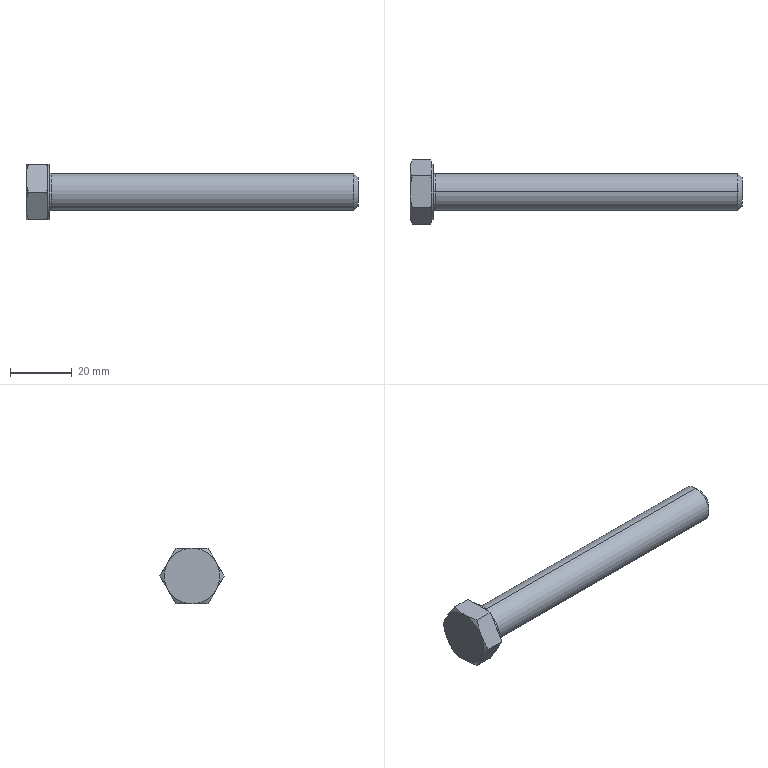Part | SolidWorks | features RevCut 4, Chamfer 1, Extrusion 1, Fillet 1, LPattern 1, Revolution 1 | 1 solid | 35 faces | box 107.5 x 20.785 x 18 mm | volume 13361 mm3 | plane 15 | cone 14 | cylinder 4 | torus 2 | commonest cylinder face diameters 12 x2 18 x2
STEP:
#1=CARTESIAN_POINT('',(8.1,0.,6.));
#2=VERTEX_POINT('',#1);
#3=CARTESIAN_POINT('',(8.1,0.,-6.));
#4=VERTEX_POINT('',#3);
#5=CARTESIAN_POINT('',(8.1,0.,0.));
#6=DIRECTION('',(1.,0.,0.));
#7=DIRECTION('',(0.,0.,-1.));
#8=AXIS2_PLACEMENT_3D('',#5,#6,#7);
#9=CIRCLE('',#8,6.);
#10=EDGE_CURVE('',#2,#4,#9,.T.);
#11=ORIENTED_EDGE('',*,*,#10,.F.);
#12=CARTESIAN_POINT('',(7.5,0.,6.6));
#13=VERTEX_POINT('',#12);
#14=CARTESIAN_POINT('',(8.1,0.,6.6));
#15=DIRECTION('',(0.,1.,0.));
#16=DIRECTION('',(0.,0.,1.));
#17=AXIS2_PLACEMENT_3D('',#14,#15,#16);
#18=CIRCLE('',#17,0.6);
#19=EDGE_CURVE('',#2,#13,#18,.T.);
#20=ORIENTED_EDGE('',*,*,#19,.T.);
#21=CARTESIAN_POINT('',(7.5,0.,-6.6));
#22=VERTEX_POINT('',#21);
#23=CARTESIAN_POINT('',(7.5,0.,0.));
#24=DIRECTION('',(-1.,0.,0.));
#25=DIRECTION('',(0.,0.,-1.));
#26=AXIS2_PLACEMENT_3D('',#23,#24,#25);
#27=CIRCLE('',#26,6.6);
#28=EDGE_CURVE('',#22,#13,#27,.T.);
#29=ORIENTED_EDGE('',*,*,#28,.F.);
#30=CARTESIAN_POINT('',(8.1,0.,-6.6));
#31=DIRECTION('',(0.,-1.,0.));
#32=DIRECTION('',(0.,0.,-1.));
#33=AXIS2_PLACEMENT_3D('',#30,#31,#32);
#34=CIRCLE('',#33,0.6);
#35=EDGE_CURVE('',#4,#22,#34,.T.);
#36=ORIENTED_EDGE('',*,*,#35,.F.);
#37=EDGE_LOOP('',(#11,#20,#29,#36));
#38=FACE_OUTER_BOUND('',#37,.T.);
#39=CARTESIAN_POINT('',(8.1,0.,0.));
#40=DIRECTION('',(1.,0.,0.));
#41=DIRECTION('',(0.,0.,-1.));
#42=AXIS2_PLACEMENT_3D('',#39,#40,#41);
#43=TOROIDAL_SURFACE('',#42,6.6,0.6);
#44=ADVANCED_FACE('',(#38),#43,.F.);
#45=CARTESIAN_POINT('',(107.5,0.,-4.6));
#46=VERTEX_POINT('',#45);
#47=CARTESIAN_POINT('',(107.5,0.,4.6));
#48=VERTEX_POINT('',#47);
#49=CARTESIAN_POINT('',(107.5,0.,0.));
#50=DIRECTION('',(1.,0.,0.));
#51=DIRECTION('',(0.,0.,1.));
#52=AXIS2_PLACEMENT_3D('',#49,#50,#51);
#53=CIRCLE('',#52,4.6);
#54=EDGE_CURVE('',#46,#48,#53,.T.);
#55=ORIENTED_EDGE('',*,*,#54,.F.);
#56=CARTESIAN_POINT('',(106.1,0.,-6.));
#57=VERTEX_POINT('',#56);
#58=CARTESIAN_POINT('',(106.1,0.,-6.));
#59=DIRECTION('',(-0.7071,0.,-0.7071));
#60=VECTOR('',#59,1000.);
#61=LINE('',#58,#60);
#62=EDGE_CURVE('',#46,#57,#61,.T.);
#63=ORIENTED_EDGE('',*,*,#62,.T.);
#64=CARTESIAN_POINT('',(106.1,0.,6.));
#65=VERTEX_POINT('',#64);
#66=CARTESIAN_POINT('',(106.1,0.,0.));
#67=DIRECTION('',(-1.,0.,0.));
#68=DIRECTION('',(0.,0.,1.));
#69=AXIS2_PLACEMENT_3D('',#66,#67,#68);
#70=CIRCLE('',#69,6.);
#71=EDGE_CURVE('',#65,#57,#70,.T.);
#72=ORIENTED_EDGE('',*,*,#71,.F.);
#73=CARTESIAN_POINT('',(106.1,0.,6.));
#74=DIRECTION('',(-0.7071,0.,0.7071));
#75=VECTOR('',#74,1000.);
#76=LINE('',#73,#75);
#77=EDGE_CURVE('',#48,#65,#76,.T.);
#78=ORIENTED_EDGE('',*,*,#77,.F.);
#79=EDGE_LOOP('',(#55,#63,#72,#78));
#80=FACE_OUTER_BOUND('',#79,.T.);
#81=CARTESIAN_POINT('',(106.1,0.,0.));
#82=DIRECTION('',(-1.,0.,0.));
#83=DIRECTION('',(0.,0.,1.));
#84=AXIS2_PLACEMENT_3D('',#81,#82,#83);
#85=CONICAL_SURFACE('',#84,6.,0.7854);
#86=ADVANCED_FACE('',(#80),#85,.T.);
#87=ORIENTED_EDGE('',*,*,#71,.T.);
#88=CARTESIAN_POINT('',(0.,0.,-6.));
#89=DIRECTION('',(-1.,0.,0.));
#90=VECTOR('',#89,1000.);
#91=LINE('',#88,#90);
#92=EDGE_CURVE('',#57,#4,#91,.T.);
#93=ORIENTED_EDGE('',*,*,#92,.T.);
#94=CARTESIAN_POINT('',(8.1,0.,0.));
#95=DIRECTION('',(1.,0.,0.));
#96=DIRECTION('',(0.,0.,-1.));
#97=AXIS2_PLACEMENT_3D('',#94,#95,#96);
#98=CIRCLE('',#97,6.);
#99=EDGE_CURVE('',#4,#2,#98,.T.);
#100=ORIENTED_EDGE('',*,*,#99,.T.);
#101=CARTESIAN_POINT('',(0.,0.,6.));
#102=DIRECTION('',(-1.,0.,0.));
#103=VECTOR('',#102,1000.);
#104=LINE('',#101,#103);
#105=EDGE_CURVE('',#65,#2,#104,.T.);
#106=ORIENTED_EDGE('',*,*,#105,.F.);
#107=EDGE_LOOP('',(#87,#93,#100,#106));
#108=FACE_OUTER_BOUND('',#107,.T.);
#109=CARTESIAN_POINT('',(0.,0.,0.));
#110=DIRECTION('',(-1.,0.,0.));
#111=DIRECTION('',(0.,0.,1.));
#112=AXIS2_PLACEMENT_3D('',#109,#110,#111);
#113=CYLINDRICAL_SURFACE('',#112,6.);
#114=ADVANCED_FACE('',(#108),#113,.T.);
#115=CARTESIAN_POINT('',(7.5,0.,-9.));
#116=VERTEX_POINT('',#115);
#117=CARTESIAN_POINT('',(7.5,0.,9.));
#118=VERTEX_POINT('',#117);
#119=CARTESIAN_POINT('',(7.5,0.,0.));
#120=DIRECTION('',(1.,0.,0.));
#121=DIRECTION('',(0.,0.,-1.));
#122=AXIS2_PLACEMENT_3D('',#119,#120,#121);
#123=CIRCLE('',#122,9.);
#124=EDGE_CURVE('',#116,#118,#123,.T.);
#125=ORIENTED_EDGE('',*,*,#124,.F.);
#126=CARTESIAN_POINT('',(6.9,0.,-9.));
#127=VERTEX_POINT('',#126);
#128=CARTESIAN_POINT('',(0.,0.,-9.));
#129=DIRECTION('',(-1.,0.,0.));
#130=VECTOR('',#129,1000.);
#131=LINE('',#128,#130);
#132=EDGE_CURVE('',#116,#127,#131,.T.);
#133=ORIENTED_EDGE('',*,*,#132,.T.);
#134=CARTESIAN_POINT('',(6.9,7.794,-4.5));
#135=VERTEX_POINT('',#134);
#136=CARTESIAN_POINT('',(6.9,0.,0.));
#137=DIRECTION('',(-1.,0.,0.));
#138=DIRECTION('',(0.,0.,1.));
#139=AXIS2_PLACEMENT_3D('',#136,#137,#138);
#140=CIRCLE('',#139,9.);
#141=EDGE_CURVE('',#135,#127,#140,.T.);
#142=ORIENTED_EDGE('',*,*,#141,.F.);
#143=CARTESIAN_POINT('',(6.9,7.794,4.5));
#144=VERTEX_POINT('',#143);
#145=CARTESIAN_POINT('',(6.9,0.,0.));
#146=DIRECTION('',(-1.,0.,0.));
#147=DIRECTION('',(0.,0.,1.));
#148=AXIS2_PLACEMENT_3D('',#145,#146,#147);
#149=CIRCLE('',#148,9.);
#150=EDGE_CURVE('',#144,#135,#149,.T.);
#151=ORIENTED_EDGE('',*,*,#150,.F.);
#152=CARTESIAN_POINT('',(6.9,0.,9.));
#153=VERTEX_POINT('',#152);
#154=CARTESIAN_POINT('',(6.9,0.,0.));
#155=DIRECTION('',(-1.,0.,0.));
#156=DIRECTION('',(0.,0.,1.));
#157=AXIS2_PLACEMENT_3D('',#154,#155,#156);
#158=CIRCLE('',#157,9.);
#159=EDGE_CURVE('',#153,#144,#158,.T.);
#160=ORIENTED_EDGE('',*,*,#159,.F.);
#161=CARTESIAN_POINT('',(0.,0.,9.));
#162=DIRECTION('',(-1.,0.,0.));
#163=VECTOR('',#162,1000.);
#164=LINE('',#161,#163);
#165=EDGE_CURVE('',#118,#153,#164,.T.);
#166=ORIENTED_EDGE('',*,*,#165,.F.);
#167=EDGE_LOOP('',(#125,#133,#142,#151,#160,#166));
#168=FACE_OUTER_BOUND('',#167,.T.);
#169=CARTESIAN_POINT('',(0.,0.,0.));
#170=DIRECTION('',(-1.,0.,0.));
#171=DIRECTION('',(0.,0.,1.));
#172=AXIS2_PLACEMENT_3D('',#169,#170,#171);
#173=CYLINDRICAL_SURFACE('',#172,9.);
#174=ADVANCED_FACE('',(#168),#173,.T.);
#175=CARTESIAN_POINT('',(6.9,5.57,-8.352));
#176=VERTEX_POINT('',#175);
#177=CARTESIAN_POINT('',(6.9,5.196,-9.));
#178=DIRECTION('',(0.,0.5,0.866));
#179=VECTOR('',#178,1000.);
#180=LINE('',#177,#179);
#181=EDGE_CURVE('',#176,#135,#180,.T.);
#182=ORIENTED_EDGE('',*,*,#181,.F.);
#183=CARTESIAN_POINT('',(6.696,5.196,-9.));
#184=VERTEX_POINT('',#183);
#185=CARTESIAN_POINT('',(6.696,5.196,-9.));
#186=CARTESIAN_POINT('',(6.768,5.321,-8.785));
#187=CARTESIAN_POINT('',(6.836,5.445,-8.569));
#188=CARTESIAN_POINT('',(6.9,5.57,-8.352));
#189=B_SPLINE_CURVE_WITH_KNOTS('',3,(#185,#186,#187,#188),.UNSPECIFIED.,.F.,.F.,(4,4),(0.000000238,0.0007696),.UNSPECIFIED.);
#190=EDGE_CURVE('',#184,#176,#189,.T.);
#191=ORIENTED_EDGE('',*,*,#190,.F.);
#192=CARTESIAN_POINT('',(0.8038,5.196,-9.));
#193=VERTEX_POINT('',#192);
#194=CARTESIAN_POINT('',(7.5,5.196,-9.));
#195=DIRECTION('',(-1.,0.,0.));
#196=VECTOR('',#195,1000.);
#197=LINE('',#194,#196);
#198=EDGE_CURVE('',#184,#193,#197,.T.);
#199=ORIENTED_EDGE('',*,*,#198,.T.);
#200=CARTESIAN_POINT('',(0.,7.794,-4.5));
#201=VERTEX_POINT('',#200);
#202=CARTESIAN_POINT('',(0.,7.794,-4.5));
#203=CARTESIAN_POINT('',(0.,7.574,-4.882));
#204=CARTESIAN_POINT('',(0.019,7.352,-5.266));
#205=CARTESIAN_POINT('',(0.09253,6.914,-6.024));
#206=CARTESIAN_POINT('',(0.147,6.697,-6.401));
#207=CARTESIAN_POINT('',(0.357,6.048,-7.525));
#208=CARTESIAN_POINT('',(0.5591,5.62,-8.266));
#209=CARTESIAN_POINT('',(0.8038,5.196,-9.));
#210=B_SPLINE_CURVE_WITH_KNOTS('',3,(#202,#203,#204,#205,#206,#207,#208,#209),.UNSPECIFIED.,.F.,.F.,(4,2,2,4),(0.005258,0.006567,0.007877,0.0105),.UNSPECIFIED.);
#211=EDGE_CURVE('',#201,#193,#210,.T.);
#212=ORIENTED_EDGE('',*,*,#211,.F.);
#213=CARTESIAN_POINT('',(0.8038,10.392,0.));
#214=VERTEX_POINT('',#213);
#215=CARTESIAN_POINT('',(0.8038,10.392,0.));
#216=CARTESIAN_POINT('',(0.5585,9.967,-0.7361));
#217=CARTESIAN_POINT('',(0.3563,9.539,-1.478));
#218=CARTESIAN_POINT('',(0.07661,8.674,-2.976));
#219=CARTESIAN_POINT('',(0.,8.237,-3.733));
#220=CARTESIAN_POINT('',(0.,7.794,-4.5));
#221=B_SPLINE_CURVE_WITH_KNOTS('',3,(#215,#216,#217,#218,#219,#220),.UNSPECIFIED.,.F.,.F.,(4,2,4),(0.000000238,0.002629,0.005258),.UNSPECIFIED.);
#222=EDGE_CURVE('',#214,#201,#221,.T.);
#223=ORIENTED_EDGE('',*,*,#222,.F.);
#224=CARTESIAN_POINT('',(6.696,10.392,0.));
#225=VERTEX_POINT('',#224);
#226=CARTESIAN_POINT('',(7.5,10.392,0.));
#227=DIRECTION('',(-1.,0.,0.));
#228=VECTOR('',#227,1000.);
#229=LINE('',#226,#228);
#230=EDGE_CURVE('',#225,#214,#229,.T.);
#231=ORIENTED_EDGE('',*,*,#230,.F.);
#232=CARTESIAN_POINT('',(6.9,10.018,-0.6478));
#233=VERTEX_POINT('',#232);
#234=CARTESIAN_POINT('',(6.9,10.018,-0.6478));
#235=CARTESIAN_POINT('',(6.836,10.143,-0.4313));
#236=CARTESIAN_POINT('',(6.768,10.268,-0.2154));
#237=CARTESIAN_POINT('',(6.696,10.392,0.));
#238=B_SPLINE_CURVE_WITH_KNOTS('',3,(#234,#235,#236,#237),.UNSPECIFIED.,.F.,.F.,(4,4),(0.009728,0.0105),.UNSPECIFIED.);
#239=EDGE_CURVE('',#233,#225,#238,.T.);
#240=ORIENTED_EDGE('',*,*,#239,.F.);
#241=CARTESIAN_POINT('',(6.9,5.196,-9.));
#242=DIRECTION('',(0.,0.5,0.866));
#243=VECTOR('',#242,1000.);
#244=LINE('',#241,#243);
#245=EDGE_CURVE('',#135,#233,#244,.T.);
#246=ORIENTED_EDGE('',*,*,#245,.F.);
#247=EDGE_LOOP('',(#182,#191,#199,#212,#223,#231,#240,#246));
#248=FACE_OUTER_BOUND('',#247,.T.);
#249=CARTESIAN_POINT('',(7.5,5.196,-9.));
#250=DIRECTION('',(0.,-0.866,0.5));
#251=DIRECTION('',(0.,-0.5,-0.866));
#252=AXIS2_PLACEMENT_3D('',#249,#250,#251);
#253=PLANE('',#252);
#254=ADVANCED_FACE('',(#248),#253,.F.);
#255=CARTESIAN_POINT('',(6.9,10.018,0.6478));
#256=VERTEX_POINT('',#255);
#257=CARTESIAN_POINT('',(6.9,10.392,0.));
#258=DIRECTION('',(0.,-0.5,0.866));
#259=VECTOR('',#258,1000.);
#260=LINE('',#257,#259);
#261=EDGE_CURVE('',#256,#144,#260,.T.);
#262=ORIENTED_EDGE('',*,*,#261,.F.);
#263=CARTESIAN_POINT('',(6.696,10.392,0.));
#264=CARTESIAN_POINT('',(6.768,10.268,0.2154));
#265=CARTESIAN_POINT('',(6.836,10.143,0.4314));
#266=CARTESIAN_POINT('',(6.9,10.018,0.6478));
#267=B_SPLINE_CURVE_WITH_KNOTS('',3,(#263,#264,#265,#266),.UNSPECIFIED.,.F.,.F.,(4,4),(0.000000238,0.0007696),.UNSPECIFIED.);
#268=EDGE_CURVE('',#225,#256,#267,.T.);
#269=ORIENTED_EDGE('',*,*,#268,.F.);
#270=ORIENTED_EDGE('',*,*,#230,.T.);
#271=CARTESIAN_POINT('',(0.,7.794,4.5));
#272=VERTEX_POINT('',#271);
#273=CARTESIAN_POINT('',(0.,7.794,4.5));
#274=CARTESIAN_POINT('',(0.,8.015,4.118));
#275=CARTESIAN_POINT('',(0.019,8.236,3.734));
#276=CARTESIAN_POINT('',(0.09253,8.674,2.976));
#277=CARTESIAN_POINT('',(0.147,8.892,2.599));
#278=CARTESIAN_POINT('',(0.357,9.541,1.475));
#279=CARTESIAN_POINT('',(0.5591,9.968,0.7343));
#280=CARTESIAN_POINT('',(0.8038,10.392,0.));
#281=B_SPLINE_CURVE_WITH_KNOTS('',3,(#273,#274,#275,#276,#277,#278,#279,#280),.UNSPECIFIED.,.F.,.F.,(4,2,2,4),(0.005258,0.006567,0.007877,0.0105),.UNSPECIFIED.);
#282=EDGE_CURVE('',#272,#214,#281,.T.);
#283=ORIENTED_EDGE('',*,*,#282,.F.);
#284=CARTESIAN_POINT('',(0.8038,5.196,9.));
#285=VERTEX_POINT('',#284);
#286=CARTESIAN_POINT('',(0.8038,5.196,9.));
#287=CARTESIAN_POINT('',(0.5585,5.621,8.264));
#288=CARTESIAN_POINT('',(0.3563,6.049,7.522));
#289=CARTESIAN_POINT('',(0.07661,6.914,6.024));
#290=CARTESIAN_POINT('',(0.,7.352,5.267));
#291=CARTESIAN_POINT('',(0.,7.794,4.5));
#292=B_SPLINE_CURVE_WITH_KNOTS('',3,(#286,#287,#288,#289,#290,#291),.UNSPECIFIED.,.F.,.F.,(4,2,4),(0.000000238,0.002629,0.005258),.UNSPECIFIED.);
#293=EDGE_CURVE('',#285,#272,#292,.T.);
#294=ORIENTED_EDGE('',*,*,#293,.F.);
#295=CARTESIAN_POINT('',(6.696,5.196,9.));
#296=VERTEX_POINT('',#295);
#297=CARTESIAN_POINT('',(7.5,5.196,9.));
#298=DIRECTION('',(-1.,0.,0.));
#299=VECTOR('',#298,1000.);
#300=LINE('',#297,#299);
#301=EDGE_CURVE('',#296,#285,#300,.T.);
#302=ORIENTED_EDGE('',*,*,#301,.F.);
#303=CARTESIAN_POINT('',(6.9,5.57,8.352));
#304=VERTEX_POINT('',#303);
#305=CARTESIAN_POINT('',(6.9,5.57,8.352));
#306=CARTESIAN_POINT('',(6.836,5.445,8.569));
#307=CARTESIAN_POINT('',(6.768,5.32,8.785));
#308=CARTESIAN_POINT('',(6.696,5.196,9.));
#309=B_SPLINE_CURVE_WITH_KNOTS('',3,(#305,#306,#307,#308),.UNSPECIFIED.,.F.,.F.,(4,4),(0.009728,0.0105),.UNSPECIFIED.);
#310=EDGE_CURVE('',#304,#296,#309,.T.);
#311=ORIENTED_EDGE('',*,*,#310,.F.);
#312=CARTESIAN_POINT('',(6.9,10.392,0.));
#313=DIRECTION('',(0.,-0.5,0.866));
#314=VECTOR('',#313,1000.);
#315=LINE('',#312,#314);
#316=EDGE_CURVE('',#144,#304,#315,.T.);
#317=ORIENTED_EDGE('',*,*,#316,.F.);
#318=EDGE_LOOP('',(#262,#269,#270,#283,#294,#302,#311,#317));
#319=FACE_OUTER_BOUND('',#318,.T.);
#320=CARTESIAN_POINT('',(7.5,10.392,0.));
#321=DIRECTION('',(0.,-0.866,-0.5));
#322=DIRECTION('',(0.,0.5,-0.866));
#323=AXIS2_PLACEMENT_3D('',#320,#321,#322);
#324=PLANE('',#323);
#325=ADVANCED_FACE('',(#319),#324,.F.);
#326=CARTESIAN_POINT('',(6.9,4.448,9.));
#327=VERTEX_POINT('',#326);
#328=CARTESIAN_POINT('',(6.9,5.196,9.));
#329=DIRECTION('',(0.,-1.,0.));
#330=VECTOR('',#329,1000.);
#331=LINE('',#328,#330);
#332=EDGE_CURVE('',#327,#153,#331,.T.);
#333=ORIENTED_EDGE('',*,*,#332,.F.);
#334=CARTESIAN_POINT('',(6.696,5.196,9.));
#335=CARTESIAN_POINT('',(6.768,4.948,9.));
#336=CARTESIAN_POINT('',(6.836,4.698,9.));
#337=CARTESIAN_POINT('',(6.9,4.448,9.));
#338=B_SPLINE_CURVE_WITH_KNOTS('',3,(#334,#335,#336,#337),.UNSPECIFIED.,.F.,.F.,(4,4),(0.02519,0.02597),.UNSPECIFIED.);
#339=EDGE_CURVE('',#296,#327,#338,.T.);
#340=ORIENTED_EDGE('',*,*,#339,.F.);
#341=ORIENTED_EDGE('',*,*,#301,.T.);
#342=CARTESIAN_POINT('',(0.,0.,9.));
#343=VERTEX_POINT('',#342);
#344=CARTESIAN_POINT('',(0.,0.,9.));
#345=CARTESIAN_POINT('',(0.,0.4401,9.));
#346=CARTESIAN_POINT('',(0.01885,0.8832,9.));
#347=CARTESIAN_POINT('',(0.09319,1.767,9.));
#348=CARTESIAN_POINT('',(0.1482,2.204,9.));
#349=CARTESIAN_POINT('',(0.3593,3.505,9.));
#350=CARTESIAN_POINT('',(0.5612,4.356,9.));
#351=CARTESIAN_POINT('',(0.8038,5.196,9.));
#352=B_SPLINE_CURVE_WITH_KNOTS('',3,(#344,#345,#346,#347,#348,#349,#350,#351),.UNSPECIFIED.,.F.,.F.,(4,2,2,4),(0.01498,0.0163,0.01761,0.02025),.UNSPECIFIED.);
#353=EDGE_CURVE('',#343,#285,#352,.T.);
#354=ORIENTED_EDGE('',*,*,#353,.F.);
#355=CARTESIAN_POINT('',(0.8038,-5.196,9.));
#356=VERTEX_POINT('',#355);
#357=CARTESIAN_POINT('',(0.8038,-5.196,9.));
#358=CARTESIAN_POINT('',(0.5595,-4.35,9.));
#359=CARTESIAN_POINT('',(0.3552,-3.485,9.));
#360=CARTESIAN_POINT('',(0.07569,-1.752,9.));
#361=CARTESIAN_POINT('',(0.,-0.8794,9.));
#362=CARTESIAN_POINT('',(0.,0.,9.));
#363=B_SPLINE_CURVE_WITH_KNOTS('',3,(#357,#358,#359,#360,#361,#362),.UNSPECIFIED.,.F.,.F.,(4,2,4),(0.00972,0.01235,0.01498),.UNSPECIFIED.);
#364=EDGE_CURVE('',#356,#343,#363,.T.);
#365=ORIENTED_EDGE('',*,*,#364,.F.);
#366=CARTESIAN_POINT('',(6.696,-5.196,9.));
#367=VERTEX_POINT('',#366);
#368=CARTESIAN_POINT('',(7.5,-5.196,9.));
#369=DIRECTION('',(-1.,0.,0.));
#370=VECTOR('',#369,1000.);
#371=LINE('',#368,#370);
#372=EDGE_CURVE('',#367,#356,#371,.T.);
#373=ORIENTED_EDGE('',*,*,#372,.F.);
#374=CARTESIAN_POINT('',(6.9,-4.448,9.));
#375=VERTEX_POINT('',#374);
#376=CARTESIAN_POINT('',(6.9,-4.448,9.));
#377=CARTESIAN_POINT('',(6.836,-4.699,9.));
#378=CARTESIAN_POINT('',(6.768,-4.948,9.));
#379=CARTESIAN_POINT('',(6.696,-5.196,9.));
#380=B_SPLINE_CURVE_WITH_KNOTS('',3,(#376,#377,#378,#379),.UNSPECIFIED.,.F.,.F.,(4,4),(0.03494,0.03571),.UNSPECIFIED.);
#381=EDGE_CURVE('',#375,#367,#380,.T.);
#382=ORIENTED_EDGE('',*,*,#381,.F.);
#383=CARTESIAN_POINT('',(6.9,5.196,9.));
#384=DIRECTION('',(0.,-1.,0.));
#385=VECTOR('',#384,1000.);
#386=LINE('',#383,#385);
#387=EDGE_CURVE('',#153,#375,#386,.T.);
#388=ORIENTED_EDGE('',*,*,#387,.F.);
#389=EDGE_LOOP('',(#333,#340,#341,#354,#365,#373,#382,#388));
#390=FACE_OUTER_BOUND('',#389,.T.);
#391=CARTESIAN_POINT('',(7.5,5.196,9.));
#392=DIRECTION('',(0.,0.,-1.));
#393=DIRECTION('',(-1.,0.,0.));
#394=AXIS2_PLACEMENT_3D('',#391,#392,#393);
#395=PLANE('',#394);
#396=ADVANCED_FACE('',(#390),#395,.F.);
#397=CARTESIAN_POINT('',(6.9,-5.57,8.352));
#398=VERTEX_POINT('',#397);
#399=CARTESIAN_POINT('',(6.9,-7.794,4.5));
#400=VERTEX_POINT('',#399);
#401=CARTESIAN_POINT('',(6.9,-10.392,0.));
#402=DIRECTION('',(0.,-0.5,-0.866));
#403=VECTOR('',#402,1000.);
#404=LINE('',#401,#403);
#405=EDGE_CURVE('',#398,#400,#404,.T.);
#406=ORIENTED_EDGE('',*,*,#405,.F.);
#407=CARTESIAN_POINT('',(6.696,-5.196,9.));
#408=CARTESIAN_POINT('',(6.768,-5.321,8.785));
#409=CARTESIAN_POINT('',(6.836,-5.445,8.569));
#410=CARTESIAN_POINT('',(6.9,-5.57,8.352));
#411=B_SPLINE_CURVE_WITH_KNOTS('',3,(#407,#408,#409,#410),.UNSPECIFIED.,.F.,.F.,(4,4),(0.000000238,0.0007696),.UNSPECIFIED.);
#412=EDGE_CURVE('',#367,#398,#411,.T.);
#413=ORIENTED_EDGE('',*,*,#412,.F.);
#414=ORIENTED_EDGE('',*,*,#372,.T.);
#415=CARTESIAN_POINT('',(0.,-7.794,4.5));
#416=VERTEX_POINT('',#415);
#417=CARTESIAN_POINT('',(0.,-7.794,4.5));
#418=CARTESIAN_POINT('',(0.,-7.574,4.882));
#419=CARTESIAN_POINT('',(0.019,-7.352,5.266));
#420=CARTESIAN_POINT('',(0.09253,-6.914,6.024));
#421=CARTESIAN_POINT('',(0.147,-6.697,6.401));
#422=CARTESIAN_POINT('',(0.357,-6.048,7.525));
#423=CARTESIAN_POINT('',(0.5591,-5.62,8.266));
#424=CARTESIAN_POINT('',(0.8038,-5.196,9.));
#425=B_SPLINE_CURVE_WITH_KNOTS('',3,(#417,#418,#419,#420,#421,#422,#423,#424),.UNSPECIFIED.,.F.,.F.,(4,2,2,4),(0.005258,0.006567,0.007877,0.0105),.UNSPECIFIED.);
#426=EDGE_CURVE('',#416,#356,#425,.T.);
#427=ORIENTED_EDGE('',*,*,#426,.F.);
#428=CARTESIAN_POINT('',(0.8038,-10.392,0.));
#429=VERTEX_POINT('',#428);
#430=CARTESIAN_POINT('',(0.8038,-10.392,0.));
#431=CARTESIAN_POINT('',(0.5585,-9.967,0.7361));
#432=CARTESIAN_POINT('',(0.3563,-9.539,1.478));
#433=CARTESIAN_POINT('',(0.07661,-8.674,2.976));
#434=CARTESIAN_POINT('',(0.,-8.237,3.733));
#435=CARTESIAN_POINT('',(0.,-7.794,4.5));
#436=B_SPLINE_CURVE_WITH_KNOTS('',3,(#430,#431,#432,#433,#434,#435),.UNSPECIFIED.,.F.,.F.,(4,2,4),(0.000000238,0.002629,0.005258),.UNSPECIFIED.);
#437=EDGE_CURVE('',#429,#416,#436,.T.);
#438=ORIENTED_EDGE('',*,*,#437,.F.);
#439=CARTESIAN_POINT('',(6.696,-10.392,0.));
#440=VERTEX_POINT('',#439);
#441=CARTESIAN_POINT('',(7.5,-10.392,0.));
#442=DIRECTION('',(-1.,0.,0.));
#443=VECTOR('',#442,1000.);
#444=LINE('',#441,#443);
#445=EDGE_CURVE('',#440,#429,#444,.T.);
#446=ORIENTED_EDGE('',*,*,#445,.F.);
#447=CARTESIAN_POINT('',(6.9,-10.018,0.6478));
#448=VERTEX_POINT('',#447);
#449=CARTESIAN_POINT('',(6.9,-10.018,0.6478));
#450=CARTESIAN_POINT('',(6.836,-10.143,0.4313));
#451=CARTESIAN_POINT('',(6.768,-10.268,0.2154));
#452=CARTESIAN_POINT('',(6.696,-10.392,0.));
#453=B_SPLINE_CURVE_WITH_KNOTS('',3,(#449,#450,#451,#452),.UNSPECIFIED.,.F.,.F.,(4,4),(0.009728,0.0105),.UNSPECIFIED.);
#454=EDGE_CURVE('',#448,#440,#453,.T.);
#455=ORIENTED_EDGE('',*,*,#454,.F.);
#456=CARTESIAN_POINT('',(6.9,-10.392,0.));
#457=DIRECTION('',(0.,-0.5,-0.866));
#458=VECTOR('',#457,1000.);
#459=LINE('',#456,#458);
#460=EDGE_CURVE('',#400,#448,#459,.T.);
#461=ORIENTED_EDGE('',*,*,#460,.F.);
#462=EDGE_LOOP('',(#406,#413,#414,#427,#438,#446,#455,#461));
#463=FACE_OUTER_BOUND('',#462,.T.);
#464=CARTESIAN_POINT('',(7.5,-10.392,0.));
#465=DIRECTION('',(0.,0.866,-0.5));
#466=DIRECTION('',(0.,0.5,0.866));
#467=AXIS2_PLACEMENT_3D('',#464,#465,#466);
#468=PLANE('',#467);
#469=ADVANCED_FACE('',(#463),#468,.F.);
#470=CARTESIAN_POINT('',(6.9,-10.018,-0.6478));
#471=VERTEX_POINT('',#470);
#472=CARTESIAN_POINT('',(6.9,-7.794,-4.5));
#473=VERTEX_POINT('',#472);
#474=CARTESIAN_POINT('',(6.9,-5.196,-9.));
#475=DIRECTION('',(0.,0.5,-0.866));
#476=VECTOR('',#475,1000.);
#477=LINE('',#474,#476);
#478=EDGE_CURVE('',#471,#473,#477,.T.);
#479=ORIENTED_EDGE('',*,*,#478,.F.);
#480=CARTESIAN_POINT('',(6.696,-10.392,0.));
#481=CARTESIAN_POINT('',(6.768,-10.268,-0.2154));
#482=CARTESIAN_POINT('',(6.836,-10.143,-0.4314));
#483=CARTESIAN_POINT('',(6.9,-10.018,-0.6478));
#484=B_SPLINE_CURVE_WITH_KNOTS('',3,(#480,#481,#482,#483),.UNSPECIFIED.,.F.,.F.,(4,4),(0.000000238,0.0007696),.UNSPECIFIED.);
#485=EDGE_CURVE('',#440,#471,#484,.T.);
#486=ORIENTED_EDGE('',*,*,#485,.F.);
#487=ORIENTED_EDGE('',*,*,#445,.T.);
#488=CARTESIAN_POINT('',(0.,-7.794,-4.5));
#489=VERTEX_POINT('',#488);
#490=CARTESIAN_POINT('',(0.,-7.794,-4.5));
#491=CARTESIAN_POINT('',(0.,-8.015,-4.118));
#492=CARTESIAN_POINT('',(0.019,-8.236,-3.734));
#493=CARTESIAN_POINT('',(0.09253,-8.674,-2.976));
#494=CARTESIAN_POINT('',(0.147,-8.892,-2.599));
#495=CARTESIAN_POINT('',(0.357,-9.541,-1.475));
#496=CARTESIAN_POINT('',(0.5591,-9.968,-0.7343));
#497=CARTESIAN_POINT('',(0.8038,-10.392,0.));
#498=B_SPLINE_CURVE_WITH_KNOTS('',3,(#490,#491,#492,#493,#494,#495,#496,#497),.UNSPECIFIED.,.F.,.F.,(4,2,2,4),(0.005258,0.006567,0.007877,0.0105),.UNSPECIFIED.);
#499=EDGE_CURVE('',#489,#429,#498,.T.);
#500=ORIENTED_EDGE('',*,*,#499,.F.);
#501=CARTESIAN_POINT('',(0.8038,-5.196,-9.));
#502=VERTEX_POINT('',#501);
#503=CARTESIAN_POINT('',(0.8038,-5.196,-9.));
#504=CARTESIAN_POINT('',(0.5585,-5.621,-8.264));
#505=CARTESIAN_POINT('',(0.3563,-6.049,-7.522));
#506=CARTESIAN_POINT('',(0.07661,-6.914,-6.024));
#507=CARTESIAN_POINT('',(0.,-7.352,-5.267));
#508=CARTESIAN_POINT('',(0.,-7.794,-4.5));
#509=B_SPLINE_CURVE_WITH_KNOTS('',3,(#503,#504,#505,#506,#507,#508),.UNSPECIFIED.,.F.,.F.,(4,2,4),(0.000000238,0.002629,0.005258),.UNSPECIFIED.);
#510=EDGE_CURVE('',#502,#489,#509,.T.);
#511=ORIENTED_EDGE('',*,*,#510,.F.);
#512=CARTESIAN_POINT('',(6.696,-5.196,-9.));
#513=VERTEX_POINT('',#512);
#514=CARTESIAN_POINT('',(7.5,-5.196,-9.));
#515=DIRECTION('',(-1.,0.,0.));
#516=VECTOR('',#515,1000.);
#517=LINE('',#514,#516);
#518=EDGE_CURVE('',#513,#502,#517,.T.);
#519=ORIENTED_EDGE('',*,*,#518,.F.);
#520=CARTESIAN_POINT('',(6.9,-5.57,-8.352));
#521=VERTEX_POINT('',#520);
#522=CARTESIAN_POINT('',(6.9,-5.57,-8.352));
#523=CARTESIAN_POINT('',(6.836,-5.445,-8.569));
#524=CARTESIAN_POINT('',(6.768,-5.32,-8.785));
#525=CARTESIAN_POINT('',(6.696,-5.196,-9.));
#526=B_SPLINE_CURVE_WITH_KNOTS('',3,(#522,#523,#524,#525),.UNSPECIFIED.,.F.,.F.,(4,4),(0.009728,0.0105),.UNSPECIFIED.);
#527=EDGE_CURVE('',#521,#513,#526,.T.);
#528=ORIENTED_EDGE('',*,*,#527,.F.);
#529=CARTESIAN_POINT('',(6.9,-5.196,-9.));
#530=DIRECTION('',(0.,0.5,-0.866));
#531=VECTOR('',#530,1000.);
#532=LINE('',#529,#531);
#533=EDGE_CURVE('',#473,#521,#532,.T.);
#534=ORIENTED_EDGE('',*,*,#533,.F.);
#535=EDGE_LOOP('',(#479,#486,#487,#500,#511,#519,#528,#534));
#536=FACE_OUTER_BOUND('',#535,.T.);
#537=CARTESIAN_POINT('',(7.5,-5.196,-9.));
#538=DIRECTION('',(0.,0.866,0.5));
#539=DIRECTION('',(0.,-0.5,0.866));
#540=AXIS2_PLACEMENT_3D('',#537,#538,#539);
#541=PLANE('',#540);
#542=ADVANCED_FACE('',(#536),#541,.F.);
#543=CARTESIAN_POINT('',(6.9,-4.448,-9.));
#544=VERTEX_POINT('',#543);
#545=CARTESIAN_POINT('',(6.9,5.196,-9.));
#546=DIRECTION('',(0.,1.,0.));
#547=VECTOR('',#546,1000.);
#548=LINE('',#545,#547);
#549=EDGE_CURVE('',#544,#127,#548,.T.);
#550=ORIENTED_EDGE('',*,*,#549,.F.);
#551=CARTESIAN_POINT('',(6.696,-5.196,-9.));
#552=CARTESIAN_POINT('',(6.768,-4.948,-9.));
#553=CARTESIAN_POINT('',(6.836,-4.699,-9.));
#554=CARTESIAN_POINT('',(6.9,-4.448,-9.));
#555=B_SPLINE_CURVE_WITH_KNOTS('',3,(#551,#552,#553,#554),.UNSPECIFIED.,.F.,.F.,(4,4),(0.00972,0.01049),.UNSPECIFIED.);
#556=EDGE_CURVE('',#513,#544,#555,.T.);
#557=ORIENTED_EDGE('',*,*,#556,.F.);
#558=ORIENTED_EDGE('',*,*,#518,.T.);
#559=CARTESIAN_POINT('',(0.,0.,-9.));
#560=VERTEX_POINT('',#559);
#561=CARTESIAN_POINT('',(0.,0.,-9.));
#562=CARTESIAN_POINT('',(0.,-0.8794,-9.));
#563=CARTESIAN_POINT('',(0.07569,-1.752,-9.));
#564=CARTESIAN_POINT('',(0.3552,-3.485,-9.));
#565=CARTESIAN_POINT('',(0.5595,-4.35,-9.));
#566=CARTESIAN_POINT('',(0.8038,-5.196,-9.));
#567=B_SPLINE_CURVE_WITH_KNOTS('',3,(#561,#562,#563,#564,#565,#566),.UNSPECIFIED.,.F.,.F.,(4,2,4),(0.03045,0.03308,0.03571),.UNSPECIFIED.);
#568=EDGE_CURVE('',#560,#502,#567,.T.);
#569=ORIENTED_EDGE('',*,*,#568,.F.);
#570=CARTESIAN_POINT('',(0.8038,5.196,-9.));
#571=CARTESIAN_POINT('',(0.5612,4.356,-9.));
#572=CARTESIAN_POINT('',(0.3593,3.505,-9.));
#573=CARTESIAN_POINT('',(0.1482,2.204,-9.));
#574=CARTESIAN_POINT('',(0.09319,1.767,-9.));
#575=CARTESIAN_POINT('',(0.01885,0.8832,-9.));
#576=CARTESIAN_POINT('',(0.,0.4401,-9.));
#577=CARTESIAN_POINT('',(0.,0.,-9.));
#578=B_SPLINE_CURVE_WITH_KNOTS('',3,(#570,#571,#572,#573,#574,#575,#576,#577),.UNSPECIFIED.,.F.,.F.,(4,2,2,4),(0.02519,0.02782,0.02914,0.03045),.UNSPECIFIED.);
#579=EDGE_CURVE('',#193,#560,#578,.T.);
#580=ORIENTED_EDGE('',*,*,#579,.F.);
#581=ORIENTED_EDGE('',*,*,#198,.F.);
#582=CARTESIAN_POINT('',(6.9,4.448,-9.));
#583=VERTEX_POINT('',#582);
#584=CARTESIAN_POINT('',(6.9,4.448,-9.));
#585=CARTESIAN_POINT('',(6.836,4.698,-9.));
#586=CARTESIAN_POINT('',(6.768,4.948,-9.));
#587=CARTESIAN_POINT('',(6.696,5.196,-9.));
#588=B_SPLINE_CURVE_WITH_KNOTS('',3,(#584,#585,#586,#587),.UNSPECIFIED.,.F.,.F.,(4,4),(0.01947,0.02025),.UNSPECIFIED.);
#589=EDGE_CURVE('',#583,#184,#588,.T.);
#590=ORIENTED_EDGE('',*,*,#589,.F.);
#591=CARTESIAN_POINT('',(6.9,5.196,-9.));
#592=DIRECTION('',(0.,1.,0.));
#593=VECTOR('',#592,1000.);
#594=LINE('',#591,#593);
#595=EDGE_CURVE('',#127,#583,#594,.T.);
#596=ORIENTED_EDGE('',*,*,#595,.F.);
#597=EDGE_LOOP('',(#550,#557,#558,#569,#580,#581,#590,#596));
#598=FACE_OUTER_BOUND('',#597,.T.);
#599=CARTESIAN_POINT('',(7.5,5.196,-9.));
#600=DIRECTION('',(0.,0.,1.));
#601=DIRECTION('',(1.,0.,0.));
#602=AXIS2_PLACEMENT_3D('',#599,#600,#601);
#603=PLANE('',#602);
#604=ADVANCED_FACE('',(#598),#603,.F.);
#605=ORIENTED_EDGE('',*,*,#556,.T.);
#606=CARTESIAN_POINT('',(6.9,0.,0.));
#607=DIRECTION('',(-1.,0.,0.));
#608=DIRECTION('',(0.,0.,-1.));
#609=AXIS2_PLACEMENT_3D('',#606,#607,#608);
#610=CIRCLE('',#609,10.039);
#611=EDGE_CURVE('',#544,#521,#610,.T.);
#612=ORIENTED_EDGE('',*,*,#611,.T.);
#613=ORIENTED_EDGE('',*,*,#527,.T.);
#614=EDGE_LOOP('',(#605,#612,#613));
#615=FACE_OUTER_BOUND('',#614,.T.);
#616=CARTESIAN_POINT('',(3.809,0.,0.));
#617=DIRECTION('',(-1.,0.,0.));
#618=DIRECTION('',(0.,0.,1.));
#619=AXIS2_PLACEMENT_3D('',#616,#617,#618);
#620=CONICAL_SURFACE('',#619,15.392,1.047);
#621=ADVANCED_FACE('',(#615),#620,.T.);
#622=ORIENTED_EDGE('',*,*,#485,.T.);
#623=CARTESIAN_POINT('',(6.9,0.,0.));
#624=DIRECTION('',(-1.,0.,0.));
#625=DIRECTION('',(0.,0.,-1.));
#626=AXIS2_PLACEMENT_3D('',#623,#624,#625);
#627=CIRCLE('',#626,10.039);
#628=EDGE_CURVE('',#471,#448,#627,.T.);
#629=ORIENTED_EDGE('',*,*,#628,.T.);
#630=ORIENTED_EDGE('',*,*,#454,.T.);
#631=EDGE_LOOP('',(#622,#629,#630));
#632=FACE_OUTER_BOUND('',#631,.T.);
#633=CARTESIAN_POINT('',(3.809,0.,0.));
#634=DIRECTION('',(-1.,0.,0.));
#635=DIRECTION('',(0.,0.,1.));
#636=AXIS2_PLACEMENT_3D('',#633,#634,#635);
#637=CONICAL_SURFACE('',#636,15.392,1.047);
#638=ADVANCED_FACE('',(#632),#637,.T.);
#639=ORIENTED_EDGE('',*,*,#412,.T.);
#640=CARTESIAN_POINT('',(6.9,0.,0.));
#641=DIRECTION('',(-1.,0.,0.));
#642=DIRECTION('',(0.,0.,-1.));
#643=AXIS2_PLACEMENT_3D('',#640,#641,#642);
#644=CIRCLE('',#643,10.039);
#645=EDGE_CURVE('',#398,#375,#644,.T.);
#646=ORIENTED_EDGE('',*,*,#645,.T.);
#647=ORIENTED_EDGE('',*,*,#381,.T.);
#648=EDGE_LOOP('',(#639,#646,#647));
#649=FACE_OUTER_BOUND('',#648,.T.);
#650=CARTESIAN_POINT('',(3.809,0.,0.));
#651=DIRECTION('',(-1.,0.,0.));
#652=DIRECTION('',(0.,0.,1.));
#653=AXIS2_PLACEMENT_3D('',#650,#651,#652);
#654=CONICAL_SURFACE('',#653,15.392,1.047);
#655=ADVANCED_FACE('',(#649),#654,.T.);
#656=ORIENTED_EDGE('',*,*,#339,.T.);
#657=CARTESIAN_POINT('',(6.9,0.,0.));
#658=DIRECTION('',(-1.,0.,0.));
#659=DIRECTION('',(0.,0.,-1.));
#660=AXIS2_PLACEMENT_3D('',#657,#658,#659);
#661=CIRCLE('',#660,10.039);
#662=EDGE_CURVE('',#327,#304,#661,.T.);
#663=ORIENTED_EDGE('',*,*,#662,.T.);
#664=ORIENTED_EDGE('',*,*,#310,.T.);
#665=EDGE_LOOP('',(#656,#663,#664));
#666=FACE_OUTER_BOUND('',#665,.T.);
#667=CARTESIAN_POINT('',(3.809,0.,0.));
#668=DIRECTION('',(-1.,0.,0.));
#669=DIRECTION('',(0.,0.,1.));
#670=AXIS2_PLACEMENT_3D('',#667,#668,#669);
#671=CONICAL_SURFACE('',#670,15.392,1.047);
#672=ADVANCED_FACE('',(#666),#671,.T.);
#673=ORIENTED_EDGE('',*,*,#268,.T.);
#674=CARTESIAN_POINT('',(6.9,0.,0.));
#675=DIRECTION('',(-1.,0.,0.));
#676=DIRECTION('',(0.,0.,-1.));
#677=AXIS2_PLACEMENT_3D('',#674,#675,#676);
#678=CIRCLE('',#677,10.039);
#679=EDGE_CURVE('',#256,#233,#678,.T.);
#680=ORIENTED_EDGE('',*,*,#679,.T.);
#681=ORIENTED_EDGE('',*,*,#239,.T.);
#682=EDGE_LOOP('',(#673,#680,#681));
#683=FACE_OUTER_BOUND('',#682,.T.);
#684=CARTESIAN_POINT('',(3.809,0.,0.));
#685=DIRECTION('',(-1.,0.,0.));
#686=DIRECTION('',(0.,0.,1.));
#687=AXIS2_PLACEMENT_3D('',#684,#685,#686);
#688=CONICAL_SURFACE('',#687,15.392,1.047);
#689=ADVANCED_FACE('',(#683),#688,.T.);
#690=ORIENTED_EDGE('',*,*,#190,.T.);
#691=CARTESIAN_POINT('',(6.9,0.,0.));
#692=DIRECTION('',(-1.,0.,0.));
#693=DIRECTION('',(0.,0.,-1.));
#694=AXIS2_PLACEMENT_3D('',#691,#692,#693);
#695=CIRCLE('',#694,10.039);
#696=EDGE_CURVE('',#176,#583,#695,.T.);
#697=ORIENTED_EDGE('',*,*,#696,.T.);
#698=ORIENTED_EDGE('',*,*,#589,.T.);
#699=EDGE_LOOP('',(#690,#697,#698));
#700=FACE_OUTER_BOUND('',#699,.T.);
#701=CARTESIAN_POINT('',(3.809,0.,0.));
#702=DIRECTION('',(-1.,0.,0.));
#703=DIRECTION('',(0.,0.,1.));
#704=AXIS2_PLACEMENT_3D('',#701,#702,#703);
#705=CONICAL_SURFACE('',#704,15.392,1.047);
#706=ADVANCED_FACE('',(#700),#705,.T.);
#707=ORIENTED_EDGE('',*,*,#510,.T.);
#708=CARTESIAN_POINT('',(0.,0.,0.));
#709=DIRECTION('',(1.,0.,0.));
#710=DIRECTION('',(0.,0.,-1.));
#711=AXIS2_PLACEMENT_3D('',#708,#709,#710);
#712=CIRCLE('',#711,9.);
#713=EDGE_CURVE('',#489,#560,#712,.T.);
#714=ORIENTED_EDGE('',*,*,#713,.T.);
#715=ORIENTED_EDGE('',*,*,#568,.T.);
#716=EDGE_LOOP('',(#707,#714,#715));
#717=FACE_OUTER_BOUND('',#716,.T.);
#718=CARTESIAN_POINT('',(0.,0.,0.));
#719=DIRECTION('',(1.,0.,0.));
#720=DIRECTION('',(0.,0.,-1.));
#721=AXIS2_PLACEMENT_3D('',#718,#719,#720);
#722=CONICAL_SURFACE('',#721,9.,1.047);
#723=ADVANCED_FACE('',(#717),#722,.T.);
#724=ORIENTED_EDGE('',*,*,#437,.T.);
#725=CARTESIAN_POINT('',(0.,0.,0.));
#726=DIRECTION('',(1.,0.,0.));
#727=DIRECTION('',(0.,0.,-1.));
#728=AXIS2_PLACEMENT_3D('',#725,#726,#727);
#729=CIRCLE('',#728,9.);
#730=EDGE_CURVE('',#416,#489,#729,.T.);
#731=ORIENTED_EDGE('',*,*,#730,.T.);
#732=ORIENTED_EDGE('',*,*,#499,.T.);
#733=EDGE_LOOP('',(#724,#731,#732));
#734=FACE_OUTER_BOUND('',#733,.T.);
#735=CARTESIAN_POINT('',(0.,0.,0.));
#736=DIRECTION('',(1.,0.,0.));
#737=DIRECTION('',(0.,0.,-1.));
#738=AXIS2_PLACEMENT_3D('',#735,#736,#737);
#739=CONICAL_SURFACE('',#738,9.,1.047);
#740=ADVANCED_FACE('',(#734),#739,.T.);
#741=ORIENTED_EDGE('',*,*,#364,.T.);
#742=CARTESIAN_POINT('',(0.,0.,0.));
#743=DIRECTION('',(1.,0.,0.));
#744=DIRECTION('',(0.,0.,-1.));
#745=AXIS2_PLACEMENT_3D('',#742,#743,#744);
#746=CIRCLE('',#745,9.);
#747=EDGE_CURVE('',#343,#416,#746,.T.);
#748=ORIENTED_EDGE('',*,*,#747,.T.);
#749=ORIENTED_EDGE('',*,*,#426,.T.);
#750=EDGE_LOOP('',(#741,#748,#749));
#751=FACE_OUTER_BOUND('',#750,.T.);
#752=CARTESIAN_POINT('',(0.,0.,0.));
#753=DIRECTION('',(1.,0.,0.));
#754=DIRECTION('',(0.,0.,-1.));
#755=AXIS2_PLACEMENT_3D('',#752,#753,#754);
#756=CONICAL_SURFACE('',#755,9.,1.047);
#757=ADVANCED_FACE('',(#751),#756,.T.);
#758=ORIENTED_EDGE('',*,*,#353,.T.);
#759=ORIENTED_EDGE('',*,*,#293,.T.);
#760=CARTESIAN_POINT('',(0.,0.,0.));
#761=DIRECTION('',(-1.,0.,0.));
#762=DIRECTION('',(0.,0.,1.));
#763=AXIS2_PLACEMENT_3D('',#760,#761,#762);
#764=CIRCLE('',#763,9.);
#765=EDGE_CURVE('',#343,#272,#764,.T.);
#766=ORIENTED_EDGE('',*,*,#765,.F.);
#767=EDGE_LOOP('',(#758,#759,#766));
#768=FACE_OUTER_BOUND('',#767,.T.);
#769=CARTESIAN_POINT('',(0.,0.,0.));
#770=DIRECTION('',(1.,0.,0.));
#771=DIRECTION('',(0.,0.,-1.));
#772=AXIS2_PLACEMENT_3D('',#769,#770,#771);
#773=CONICAL_SURFACE('',#772,9.,1.047);
#774=ADVANCED_FACE('',(#768),#773,.T.);
#775=ORIENTED_EDGE('',*,*,#282,.T.);
#776=ORIENTED_EDGE('',*,*,#222,.T.);
#777=CARTESIAN_POINT('',(0.,0.,0.));
#778=DIRECTION('',(1.,0.,0.));
#779=DIRECTION('',(0.,0.,-1.));
#780=AXIS2_PLACEMENT_3D('',#777,#778,#779);
#781=CIRCLE('',#780,9.);
#782=EDGE_CURVE('',#201,#272,#781,.T.);
#783=ORIENTED_EDGE('',*,*,#782,.T.);
#784=EDGE_LOOP('',(#775,#776,#783));
#785=FACE_OUTER_BOUND('',#784,.T.);
#786=CARTESIAN_POINT('',(0.,0.,0.));
#787=DIRECTION('',(1.,0.,0.));
#788=DIRECTION('',(0.,0.,-1.));
#789=AXIS2_PLACEMENT_3D('',#786,#787,#788);
#790=CONICAL_SURFACE('',#789,9.,1.047);
#791=ADVANCED_FACE('',(#785),#790,.T.);
#792=ORIENTED_EDGE('',*,*,#211,.T.);
#793=ORIENTED_EDGE('',*,*,#579,.T.);
#794=CARTESIAN_POINT('',(0.,0.,0.));
#795=DIRECTION('',(1.,0.,0.));
#796=DIRECTION('',(0.,0.,-1.));
#797=AXIS2_PLACEMENT_3D('',#794,#795,#796);
#798=CIRCLE('',#797,9.);
#799=EDGE_CURVE('',#560,#201,#798,.T.);
#800=ORIENTED_EDGE('',*,*,#799,.T.);
#801=EDGE_LOOP('',(#792,#793,#800));
#802=FACE_OUTER_BOUND('',#801,.T.);
#803=CARTESIAN_POINT('',(0.,0.,0.));
#804=DIRECTION('',(1.,0.,0.));
#805=DIRECTION('',(0.,0.,-1.));
#806=AXIS2_PLACEMENT_3D('',#803,#804,#805);
#807=CONICAL_SURFACE('',#806,9.,1.047);
#808=ADVANCED_FACE('',(#802),#807,.T.);
#809=ORIENTED_EDGE('',*,*,#799,.F.);
#810=ORIENTED_EDGE('',*,*,#713,.F.);
#811=ORIENTED_EDGE('',*,*,#730,.F.);
#812=ORIENTED_EDGE('',*,*,#747,.F.);
#813=ORIENTED_EDGE('',*,*,#765,.T.);
#814=ORIENTED_EDGE('',*,*,#782,.F.);
#815=EDGE_LOOP('',(#809,#810,#811,#812,#813,#814));
#816=FACE_OUTER_BOUND('',#815,.T.);
#817=CARTESIAN_POINT('',(0.,10.392,0.));
#818=DIRECTION('',(1.,0.,0.));
#819=DIRECTION('',(0.,0.,-1.));
#820=AXIS2_PLACEMENT_3D('',#817,#818,#819);
#821=PLANE('',#820);
#822=ADVANCED_FACE('',(#816),#821,.F.);
#823=ORIENTED_EDGE('',*,*,#387,.T.);
#824=ORIENTED_EDGE('',*,*,#645,.F.);
#825=ORIENTED_EDGE('',*,*,#405,.T.);
#826=CARTESIAN_POINT('',(6.9,0.,0.));
#827=DIRECTION('',(-1.,0.,0.));
#828=DIRECTION('',(0.,0.,1.));
#829=AXIS2_PLACEMENT_3D('',#826,#827,#828);
#830=CIRCLE('',#829,9.);
#831=EDGE_CURVE('',#400,#153,#830,.T.);
#832=ORIENTED_EDGE('',*,*,#831,.T.);
#833=EDGE_LOOP('',(#823,#824,#825,#832));
#834=FACE_OUTER_BOUND('',#833,.T.);
#835=CARTESIAN_POINT('',(6.9,9.,0.));
#836=DIRECTION('',(1.,0.,0.));
#837=DIRECTION('',(0.,0.,-1.));
#838=AXIS2_PLACEMENT_3D('',#835,#836,#837);
#839=PLANE('',#838);
#840=ADVANCED_FACE('',(#834),#839,.T.);
#841=ORIENTED_EDGE('',*,*,#261,.T.);
#842=ORIENTED_EDGE('',*,*,#150,.T.);
#843=ORIENTED_EDGE('',*,*,#245,.T.);
#844=ORIENTED_EDGE('',*,*,#679,.F.);
#845=EDGE_LOOP('',(#841,#842,#843,#844));
#846=FACE_OUTER_BOUND('',#845,.T.);
#847=CARTESIAN_POINT('',(6.9,9.,0.));
#848=DIRECTION('',(1.,0.,0.));
#849=DIRECTION('',(0.,0.,-1.));
#850=AXIS2_PLACEMENT_3D('',#847,#848,#849);
#851=PLANE('',#850);
#852=ADVANCED_FACE('',(#846),#851,.T.);
#853=ORIENTED_EDGE('',*,*,#460,.T.);
#854=ORIENTED_EDGE('',*,*,#628,.F.);
#855=ORIENTED_EDGE('',*,*,#478,.T.);
#856=CARTESIAN_POINT('',(6.9,0.,0.));
#857=DIRECTION('',(-1.,0.,0.));
#858=DIRECTION('',(0.,0.,1.));
#859=AXIS2_PLACEMENT_3D('',#856,#857,#858);
#860=CIRCLE('',#859,9.);
#861=EDGE_CURVE('',#473,#400,#860,.T.);
#862=ORIENTED_EDGE('',*,*,#861,.T.);
#863=EDGE_LOOP('',(#853,#854,#855,#862));
#864=FACE_OUTER_BOUND('',#863,.T.);
#865=CARTESIAN_POINT('',(6.9,9.,0.));
#866=DIRECTION('',(1.,0.,0.));
#867=DIRECTION('',(0.,0.,-1.));
#868=AXIS2_PLACEMENT_3D('',#865,#866,#867);
#869=PLANE('',#868);
#870=ADVANCED_FACE('',(#864),#869,.T.);
#871=ORIENTED_EDGE('',*,*,#533,.T.);
#872=ORIENTED_EDGE('',*,*,#611,.F.);
#873=ORIENTED_EDGE('',*,*,#549,.T.);
#874=CARTESIAN_POINT('',(6.9,0.,0.));
#875=DIRECTION('',(-1.,0.,0.));
#876=DIRECTION('',(0.,0.,1.));
#877=AXIS2_PLACEMENT_3D('',#874,#875,#876);
#878=CIRCLE('',#877,9.);
#879=EDGE_CURVE('',#127,#473,#878,.T.);
#880=ORIENTED_EDGE('',*,*,#879,.T.);
#881=EDGE_LOOP('',(#871,#872,#873,#880));
#882=FACE_OUTER_BOUND('',#881,.T.);
#883=CARTESIAN_POINT('',(6.9,9.,0.));
#884=DIRECTION('',(1.,0.,0.));
#885=DIRECTION('',(0.,0.,-1.));
#886=AXIS2_PLACEMENT_3D('',#883,#884,#885);
#887=PLANE('',#886);
#888=ADVANCED_FACE('',(#882),#887,.T.);
#889=ORIENTED_EDGE('',*,*,#181,.T.);
#890=ORIENTED_EDGE('',*,*,#141,.T.);
#891=ORIENTED_EDGE('',*,*,#595,.T.);
#892=ORIENTED_EDGE('',*,*,#696,.F.);
#893=EDGE_LOOP('',(#889,#890,#891,#892));
#894=FACE_OUTER_BOUND('',#893,.T.);
#895=CARTESIAN_POINT('',(6.9,9.,0.));
#896=DIRECTION('',(1.,0.,0.));
#897=DIRECTION('',(0.,0.,-1.));
#898=AXIS2_PLACEMENT_3D('',#895,#896,#897);
#899=PLANE('',#898);
#900=ADVANCED_FACE('',(#894),#899,.T.);
#901=ORIENTED_EDGE('',*,*,#132,.F.);
#902=CARTESIAN_POINT('',(7.5,0.,0.));
#903=DIRECTION('',(1.,0.,0.));
#904=DIRECTION('',(0.,0.,-1.));
#905=AXIS2_PLACEMENT_3D('',#902,#903,#904);
#906=CIRCLE('',#905,9.);
#907=EDGE_CURVE('',#118,#116,#906,.T.);
#908=ORIENTED_EDGE('',*,*,#907,.F.);
#909=ORIENTED_EDGE('',*,*,#165,.T.);
#910=ORIENTED_EDGE('',*,*,#831,.F.);
#911=ORIENTED_EDGE('',*,*,#861,.F.);
#912=ORIENTED_EDGE('',*,*,#879,.F.);
#913=EDGE_LOOP('',(#901,#908,#909,#910,#911,#912));
#914=FACE_OUTER_BOUND('',#913,.T.);
#915=CARTESIAN_POINT('',(0.,0.,0.));
#916=DIRECTION('',(-1.,0.,0.));
#917=DIRECTION('',(0.,0.,1.));
#918=AXIS2_PLACEMENT_3D('',#915,#916,#917);
#919=CYLINDRICAL_SURFACE('',#918,9.);
#920=ADVANCED_FACE('',(#914),#919,.T.);
#921=ORIENTED_EDGE('',*,*,#332,.T.);
#922=ORIENTED_EDGE('',*,*,#159,.T.);
#923=ORIENTED_EDGE('',*,*,#316,.T.);
#924=ORIENTED_EDGE('',*,*,#662,.F.);
#925=EDGE_LOOP('',(#921,#922,#923,#924));
#926=FACE_OUTER_BOUND('',#925,.T.);
#927=CARTESIAN_POINT('',(6.9,9.,0.));
#928=DIRECTION('',(1.,0.,0.));
#929=DIRECTION('',(0.,0.,-1.));
#930=AXIS2_PLACEMENT_3D('',#927,#928,#929);
#931=PLANE('',#930);
#932=ADVANCED_FACE('',(#926),#931,.T.);
#933=CARTESIAN_POINT('',(107.5,0.,0.));
#934=DIRECTION('',(1.,0.,0.));
#935=DIRECTION('',(0.,0.,1.));
#936=AXIS2_PLACEMENT_3D('',#933,#934,#935);
#937=CIRCLE('',#936,4.6);
#938=EDGE_CURVE('',#48,#46,#937,.T.);
#939=ORIENTED_EDGE('',*,*,#938,.T.);
#940=ORIENTED_EDGE('',*,*,#54,.T.);
#941=EDGE_LOOP('',(#939,#940));
#942=FACE_OUTER_BOUND('',#941,.T.);
#943=CARTESIAN_POINT('',(107.5,0.,0.));
#944=DIRECTION('',(-1.,0.,0.));
#945=DIRECTION('',(0.,0.,1.));
#946=AXIS2_PLACEMENT_3D('',#943,#944,#945);
#947=PLANE('',#946);
#948=ADVANCED_FACE('',(#942),#947,.F.);
#949=ORIENTED_EDGE('',*,*,#92,.F.);
#950=CARTESIAN_POINT('',(106.1,0.,0.));
#951=DIRECTION('',(-1.,0.,0.));
#952=DIRECTION('',(0.,0.,1.));
#953=AXIS2_PLACEMENT_3D('',#950,#951,#952);
#954=CIRCLE('',#953,6.);
#955=EDGE_CURVE('',#57,#65,#954,.T.);
#956=ORIENTED_EDGE('',*,*,#955,.T.);
#957=ORIENTED_EDGE('',*,*,#105,.T.);
#958=ORIENTED_EDGE('',*,*,#10,.T.);
#959=EDGE_LOOP('',(#949,#956,#957,#958));
#960=FACE_OUTER_BOUND('',#959,.T.);
#961=CARTESIAN_POINT('',(0.,0.,0.));
#962=DIRECTION('',(-1.,0.,0.));
#963=DIRECTION('',(0.,0.,1.));
#964=AXIS2_PLACEMENT_3D('',#961,#962,#963);
#965=CYLINDRICAL_SURFACE('',#964,6.);
#966=ADVANCED_FACE('',(#960),#965,.T.);
#967=ORIENTED_EDGE('',*,*,#28,.T.);
#968=CARTESIAN_POINT('',(7.5,0.,0.));
#969=DIRECTION('',(-1.,0.,0.));
#970=DIRECTION('',(0.,0.,-1.));
#971=AXIS2_PLACEMENT_3D('',#968,#969,#970);
#972=CIRCLE('',#971,6.6);
#973=EDGE_CURVE('',#13,#22,#972,.T.);
#974=ORIENTED_EDGE('',*,*,#973,.T.);
#975=EDGE_LOOP('',(#967,#974));
#976=FACE_BOUND('',#975,.T.);
#977=ORIENTED_EDGE('',*,*,#907,.T.);
#978=ORIENTED_EDGE('',*,*,#124,.T.);
#979=EDGE_LOOP('',(#977,#978));
#980=FACE_OUTER_BOUND('',#979,.T.);
#981=CARTESIAN_POINT('',(7.5,10.392,0.));
#982=DIRECTION('',(1.,0.,0.));
#983=DIRECTION('',(0.,0.,-1.));
#984=AXIS2_PLACEMENT_3D('',#981,#982,#983);
#985=PLANE('',#984);
#986=ADVANCED_FACE('',(#976,#980),#985,.T.);
#987=ORIENTED_EDGE('',*,*,#62,.F.);
#988=ORIENTED_EDGE('',*,*,#938,.F.);
#989=ORIENTED_EDGE('',*,*,#77,.T.);
#990=ORIENTED_EDGE('',*,*,#955,.F.);
#991=EDGE_LOOP('',(#987,#988,#989,#990));
#992=FACE_OUTER_BOUND('',#991,.T.);
#993=CARTESIAN_POINT('',(106.1,0.,0.));
#994=DIRECTION('',(-1.,0.,0.));
#995=DIRECTION('',(0.,0.,1.));
#996=AXIS2_PLACEMENT_3D('',#993,#994,#995);
#997=CONICAL_SURFACE('',#996,6.,0.7854);
#998=ADVANCED_FACE('',(#992),#997,.T.);
#999=ORIENTED_EDGE('',*,*,#19,.F.);
#1000=ORIENTED_EDGE('',*,*,#99,.F.);
#1001=ORIENTED_EDGE('',*,*,#35,.T.);
#1002=ORIENTED_EDGE('',*,*,#973,.F.);
#1003=EDGE_LOOP('',(#999,#1000,#1001,#1002));
#1004=FACE_OUTER_BOUND('',#1003,.T.);
#1005=CARTESIAN_POINT('',(8.1,0.,0.));
#1006=DIRECTION('',(1.,0.,0.));
#1007=DIRECTION('',(0.,0.,-1.));
#1008=AXIS2_PLACEMENT_3D('',#1005,#1006,#1007);
#1009=TOROIDAL_SURFACE('',#1008,6.6,0.6);
#1010=ADVANCED_FACE('',(#1004),#1009,.F.);
#1011=CLOSED_SHELL('',(#44,#86,#114,#174,#254,#325,#396,#469,#542,#604,#621,#638,#655,#672,#689,#706,#723,#740,#757,#774,#791,#808,#822,#840,#852,#870,#888,#900,#920,#932,#948,#966,#986,#998,#1010));
#1012=MANIFOLD_SOLID_BREP('',#1011);
#1013=CARTESIAN_POINT('',(0.,0.,0.));
#1014=DIRECTION('',(0.,0.,1.));
#1015=DIRECTION('',(1.,0.,0.));
#1016=AXIS2_PLACEMENT_3D('',#1013,#1014,#1015);
#1017=(LENGTH_UNIT()NAMED_UNIT(*)SI_UNIT(.MILLI.,.METRE.));
#1018=UNCERTAINTY_MEASURE_WITH_UNIT(LENGTH_MEASURE(0.00001),#1017,'','');
#1019=(NAMED_UNIT(*)PLANE_ANGLE_UNIT()SI_UNIT($,.RADIAN.));
#1020=(NAMED_UNIT(*)SI_UNIT($,.STERADIAN.)SOLID_ANGLE_UNIT());
#1021=(GEOMETRIC_REPRESENTATION_CONTEXT(3)GLOBAL_UNCERTAINTY_ASSIGNED_CONTEXT((#1018))GLOBAL_UNIT_ASSIGNED_CONTEXT((#1017,#1019,#1020))REPRESENTATION_CONTEXT('',''));
#1022=ADVANCED_BREP_SHAPE_REPRESENTATION('',(#1012,#1016),#1021);